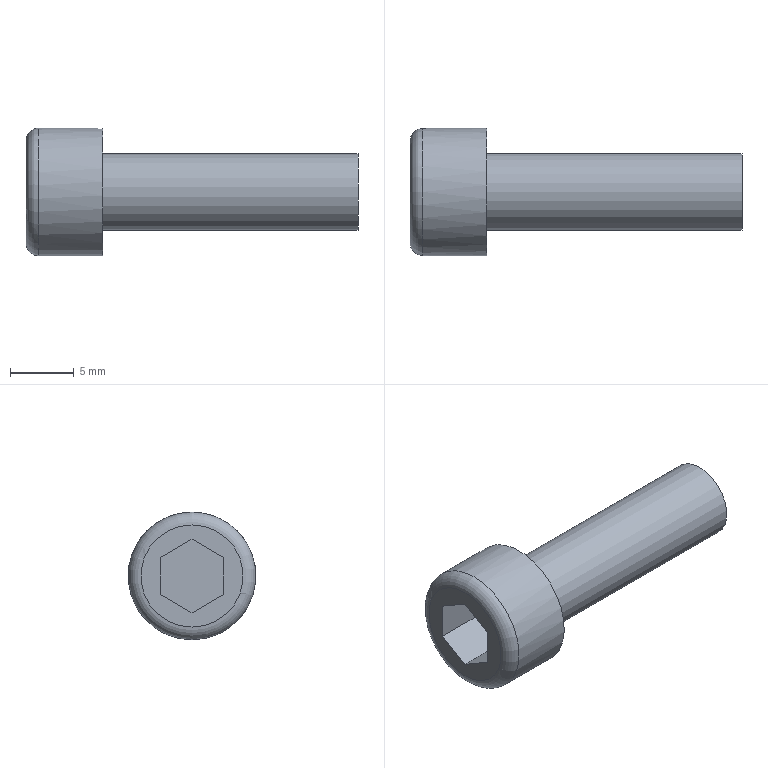Part | STEP file | Tube necking machine_id226_x_t | 1 solid | 13 faces | box 26 x 10 x 10 mm | volume 944.548 mm3 | plane 10 | cylinder 2 | torus 1 | commonest cylinder face diameters 6 x1 10 x1
STEP:
#1=CARTESIAN_POINT('',(0.,0.,0.));
#2=DIRECTION('',(0.,0.,1.));
#3=DIRECTION('',(1.,0.,0.));
#4=AXIS2_PLACEMENT_3D('',#1,#2,#3);
#5=CARTESIAN_POINT('',(-132.5,-117.,264.));
#6=VERTEX_POINT('',#5);
#7=CARTESIAN_POINT('',(-132.5,-117.,260.));
#8=DIRECTION('',(-1.,0.,0.));
#9=DIRECTION('',(0.,0.,1.));
#10=AXIS2_PLACEMENT_3D('',#7,#8,#9);
#11=CIRCLE('',#10,4.);
#12=CARTESIAN_POINT('',(-132.5,-117.,255.));
#13=DIRECTION('',(1.,0.,0.));
#14=DIRECTION('',(0.,0.,1.));
#15=AXIS2_PLACEMENT_3D('',#12,#13,#14);
#16=PLANE('',#15);
#17=CARTESIAN_POINT('',(9.,0.));
#18=CARTESIAN_POINT('',(9.,-6.928));
#19=CARTESIAN_POINT('',(3.,-3.464));
#20=CARTESIAN_POINT('',(-3.,0.));
#21=CARTESIAN_POINT('',(3.,3.464));
#22=CARTESIAN_POINT('',(9.,6.928));
#23=CARTESIAN_POINT('',(9.,0.));
#24=(BOUNDED_CURVE()B_SPLINE_CURVE(2,(#17,#18,#19,#20,#21,#22,#23),.UNSPECIFIED.,.T.,.F.)B_SPLINE_CURVE_WITH_KNOTS((1,2,2,2,2,1),(-2.094,0.,2.094,4.189,6.283,8.378),.UNSPECIFIED.)CURVE()GEOMETRIC_REPRESENTATION_ITEM()RATIONAL_B_SPLINE_CURVE((1.,0.5,1.,0.5,1.,0.5,1.))REPRESENTATION_ITEM(''));
#25=(GEOMETRIC_REPRESENTATION_CONTEXT(2)PARAMETRIC_REPRESENTATION_CONTEXT()REPRESENTATION_CONTEXT('',''));
#26=DEFINITIONAL_REPRESENTATION('',(#24),#25);
#27=PCURVE('',#16,#26);
#28=CARTESIAN_POINT('',(-131.5,-117.,260.));
#29=DIRECTION('',(1.,0.,0.));
#30=DIRECTION('',(0.,0.,1.));
#31=AXIS2_PLACEMENT_3D('',#28,#29,#30);
#32=TOROIDAL_SURFACE('',#31,4.,1.);
#33=CARTESIAN_POINT('',(6.283,4.712));
#34=DIRECTION('',(-1.,0.));
#35=VECTOR('',#34,1.);
#36=LINE('',#33,#35);
#37=(GEOMETRIC_REPRESENTATION_CONTEXT(2)PARAMETRIC_REPRESENTATION_CONTEXT()REPRESENTATION_CONTEXT('',''));
#38=DEFINITIONAL_REPRESENTATION('',(#36),#37);
#39=PCURVE('',#32,#38);
#40=SURFACE_CURVE('',#11,(#27,#39),.PCURVE_S1.);
#41=EDGE_CURVE('',#6,#6,#40,.T.);
#42=ORIENTED_EDGE('',*,*,#41,.T.);
#43=EDGE_LOOP('',(#42));
#44=FACE_BOUND('',#43,.T.);
#45=CARTESIAN_POINT('',(-132.5,-114.5,258.557));
#46=VERTEX_POINT('',#45);
#47=CARTESIAN_POINT('',(-132.5,-114.5,261.443));
#48=VERTEX_POINT('',#47);
#49=CARTESIAN_POINT('',(-132.5,-114.5,261.443));
#50=DIRECTION('',(0.,0.,1.));
#51=VECTOR('',#50,1.);
#52=LINE('',#49,#51);
#53=CARTESIAN_POINT('',(6.443,-2.5));
#54=DIRECTION('',(1.,0.));
#55=VECTOR('',#54,1.);
#56=LINE('',#53,#55);
#57=(GEOMETRIC_REPRESENTATION_CONTEXT(2)PARAMETRIC_REPRESENTATION_CONTEXT()REPRESENTATION_CONTEXT('',''));
#58=DEFINITIONAL_REPRESENTATION('',(#56),#57);
#59=PCURVE('',#16,#58);
#60=CARTESIAN_POINT('',(-128.54,-114.5,261.443));
#61=DIRECTION('',(0.,-1.,0.));
#62=DIRECTION('',(1.,0.,0.));
#63=AXIS2_PLACEMENT_3D('',#60,#61,#62);
#64=PLANE('',#63);
#65=CARTESIAN_POINT('',(-3.96,0.));
#66=DIRECTION('',(0.,1.));
#67=VECTOR('',#66,1.);
#68=LINE('',#65,#67);
#69=(GEOMETRIC_REPRESENTATION_CONTEXT(2)PARAMETRIC_REPRESENTATION_CONTEXT()REPRESENTATION_CONTEXT('',''));
#70=DEFINITIONAL_REPRESENTATION('',(#68),#69);
#71=PCURVE('',#64,#70);
#72=SURFACE_CURVE('',#52,(#59,#71),.PCURVE_S1.);
#73=EDGE_CURVE('',#46,#48,#72,.T.);
#74=ORIENTED_EDGE('',*,*,#73,.T.);
#75=CARTESIAN_POINT('',(-132.5,-117.,262.887));
#76=VERTEX_POINT('',#75);
#77=CARTESIAN_POINT('',(-132.5,-117.,262.887));
#78=DIRECTION('',(0.,-0.866,0.5));
#79=VECTOR('',#78,1.);
#80=LINE('',#77,#79);
#81=CARTESIAN_POINT('',(7.887,0.));
#82=DIRECTION('',(0.5,0.866));
#83=VECTOR('',#82,1.);
#84=LINE('',#81,#83);
#85=(GEOMETRIC_REPRESENTATION_CONTEXT(2)PARAMETRIC_REPRESENTATION_CONTEXT()REPRESENTATION_CONTEXT('',''));
#86=DEFINITIONAL_REPRESENTATION('',(#84),#85);
#87=PCURVE('',#16,#86);
#88=CARTESIAN_POINT('',(-128.54,-117.,262.887));
#89=DIRECTION('',(0.,-0.5,-0.866));
#90=DIRECTION('',(0.,0.866,-0.5));
#91=AXIS2_PLACEMENT_3D('',#88,#89,#90);
#92=PLANE('',#91);
#93=CARTESIAN_POINT('',(0.,-3.96));
#94=DIRECTION('',(-1.,0.));
#95=VECTOR('',#94,1.);
#96=LINE('',#93,#95);
#97=(GEOMETRIC_REPRESENTATION_CONTEXT(2)PARAMETRIC_REPRESENTATION_CONTEXT()REPRESENTATION_CONTEXT('',''));
#98=DEFINITIONAL_REPRESENTATION('',(#96),#97);
#99=PCURVE('',#92,#98);
#100=SURFACE_CURVE('',#80,(#87,#99),.PCURVE_S1.);
#101=EDGE_CURVE('',#48,#76,#100,.T.);
#102=ORIENTED_EDGE('',*,*,#101,.T.);
#103=CARTESIAN_POINT('',(-132.5,-119.5,261.443));
#104=VERTEX_POINT('',#103);
#105=CARTESIAN_POINT('',(-132.5,-119.5,261.443));
#106=DIRECTION('',(0.,-0.866,-0.5));
#107=VECTOR('',#106,1.);
#108=LINE('',#105,#107);
#109=CARTESIAN_POINT('',(6.443,2.5));
#110=DIRECTION('',(-0.5,0.866));
#111=VECTOR('',#110,1.);
#112=LINE('',#109,#111);
#113=(GEOMETRIC_REPRESENTATION_CONTEXT(2)PARAMETRIC_REPRESENTATION_CONTEXT()REPRESENTATION_CONTEXT('',''));
#114=DEFINITIONAL_REPRESENTATION('',(#112),#113);
#115=PCURVE('',#16,#114);
#116=CARTESIAN_POINT('',(-128.54,-119.5,261.443));
#117=DIRECTION('',(0.,0.5,-0.866));
#118=DIRECTION('',(0.,0.866,0.5));
#119=AXIS2_PLACEMENT_3D('',#116,#117,#118);
#120=PLANE('',#119);
#121=CARTESIAN_POINT('',(0.,-3.96));
#122=DIRECTION('',(-1.,0.));
#123=VECTOR('',#122,1.);
#124=LINE('',#121,#123);
#125=(GEOMETRIC_REPRESENTATION_CONTEXT(2)PARAMETRIC_REPRESENTATION_CONTEXT()REPRESENTATION_CONTEXT('',''));
#126=DEFINITIONAL_REPRESENTATION('',(#124),#125);
#127=PCURVE('',#120,#126);
#128=SURFACE_CURVE('',#108,(#115,#127),.PCURVE_S1.);
#129=EDGE_CURVE('',#76,#104,#128,.T.);
#130=ORIENTED_EDGE('',*,*,#129,.T.);
#131=CARTESIAN_POINT('',(-132.5,-119.5,258.557));
#132=VERTEX_POINT('',#131);
#133=CARTESIAN_POINT('',(-132.5,-119.5,258.557));
#134=DIRECTION('',(0.,0.,-1.));
#135=VECTOR('',#134,1.);
#136=LINE('',#133,#135);
#137=CARTESIAN_POINT('',(3.557,2.5));
#138=DIRECTION('',(-1.,0.));
#139=VECTOR('',#138,1.);
#140=LINE('',#137,#139);
#141=(GEOMETRIC_REPRESENTATION_CONTEXT(2)PARAMETRIC_REPRESENTATION_CONTEXT()REPRESENTATION_CONTEXT('',''));
#142=DEFINITIONAL_REPRESENTATION('',(#140),#141);
#143=PCURVE('',#16,#142);
#144=CARTESIAN_POINT('',(-128.54,-119.5,258.557));
#145=DIRECTION('',(0.,1.,0.));
#146=DIRECTION('',(0.,0.,1.));
#147=AXIS2_PLACEMENT_3D('',#144,#145,#146);
#148=PLANE('',#147);
#149=CARTESIAN_POINT('',(0.,-3.96));
#150=DIRECTION('',(-1.,0.));
#151=VECTOR('',#150,1.);
#152=LINE('',#149,#151);
#153=(GEOMETRIC_REPRESENTATION_CONTEXT(2)PARAMETRIC_REPRESENTATION_CONTEXT()REPRESENTATION_CONTEXT('',''));
#154=DEFINITIONAL_REPRESENTATION('',(#152),#153);
#155=PCURVE('',#148,#154);
#156=SURFACE_CURVE('',#136,(#143,#155),.PCURVE_S1.);
#157=EDGE_CURVE('',#104,#132,#156,.T.);
#158=ORIENTED_EDGE('',*,*,#157,.T.);
#159=CARTESIAN_POINT('',(-132.5,-117.,257.113));
#160=VERTEX_POINT('',#159);
#161=CARTESIAN_POINT('',(-132.5,-117.,257.113));
#162=DIRECTION('',(0.,0.866,-0.5));
#163=VECTOR('',#162,1.);
#164=LINE('',#161,#163);
#165=CARTESIAN_POINT('',(2.113,0.));
#166=DIRECTION('',(-0.5,-0.866));
#167=VECTOR('',#166,1.);
#168=LINE('',#165,#167);
#169=(GEOMETRIC_REPRESENTATION_CONTEXT(2)PARAMETRIC_REPRESENTATION_CONTEXT()REPRESENTATION_CONTEXT('',''));
#170=DEFINITIONAL_REPRESENTATION('',(#168),#169);
#171=PCURVE('',#16,#170);
#172=CARTESIAN_POINT('',(-128.54,-117.,257.113));
#173=DIRECTION('',(0.,0.5,0.866));
#174=DIRECTION('',(0.,-0.866,0.5));
#175=AXIS2_PLACEMENT_3D('',#172,#173,#174);
#176=PLANE('',#175);
#177=CARTESIAN_POINT('',(0.,-3.96));
#178=DIRECTION('',(-1.,0.));
#179=VECTOR('',#178,1.);
#180=LINE('',#177,#179);
#181=(GEOMETRIC_REPRESENTATION_CONTEXT(2)PARAMETRIC_REPRESENTATION_CONTEXT()REPRESENTATION_CONTEXT('',''));
#182=DEFINITIONAL_REPRESENTATION('',(#180),#181);
#183=PCURVE('',#176,#182);
#184=SURFACE_CURVE('',#164,(#171,#183),.PCURVE_S1.);
#185=EDGE_CURVE('',#132,#160,#184,.T.);
#186=ORIENTED_EDGE('',*,*,#185,.T.);
#187=CARTESIAN_POINT('',(-132.5,-114.5,258.557));
#188=DIRECTION('',(0.,0.866,0.5));
#189=VECTOR('',#188,1.);
#190=LINE('',#187,#189);
#191=CARTESIAN_POINT('',(3.557,-2.5));
#192=DIRECTION('',(0.5,-0.866));
#193=VECTOR('',#192,1.);
#194=LINE('',#191,#193);
#195=(GEOMETRIC_REPRESENTATION_CONTEXT(2)PARAMETRIC_REPRESENTATION_CONTEXT()REPRESENTATION_CONTEXT('',''));
#196=DEFINITIONAL_REPRESENTATION('',(#194),#195);
#197=PCURVE('',#16,#196);
#198=CARTESIAN_POINT('',(-128.54,-114.5,258.557));
#199=DIRECTION('',(0.,-0.5,0.866));
#200=DIRECTION('',(0.,-0.866,-0.5));
#201=AXIS2_PLACEMENT_3D('',#198,#199,#200);
#202=PLANE('',#201);
#203=CARTESIAN_POINT('',(0.,-3.96));
#204=DIRECTION('',(-1.,0.));
#205=VECTOR('',#204,1.);
#206=LINE('',#203,#205);
#207=(GEOMETRIC_REPRESENTATION_CONTEXT(2)PARAMETRIC_REPRESENTATION_CONTEXT()REPRESENTATION_CONTEXT('',''));
#208=DEFINITIONAL_REPRESENTATION('',(#206),#207);
#209=PCURVE('',#202,#208);
#210=SURFACE_CURVE('',#190,(#197,#209),.PCURVE_S1.);
#211=EDGE_CURVE('',#160,#46,#210,.T.);
#212=ORIENTED_EDGE('',*,*,#211,.T.);
#213=EDGE_LOOP('',(#74,#102,#130,#158,#186,#212));
#214=FACE_BOUND('',#213,.T.);
#215=ADVANCED_FACE('',(#44,#214),#16,.F.);
#216=CARTESIAN_POINT('',(-131.5,-117.,265.));
#217=VERTEX_POINT('',#216);
#218=CARTESIAN_POINT('',(-131.5,-117.,255.));
#219=VERTEX_POINT('',#218);
#220=CARTESIAN_POINT('',(-131.5,-117.,260.));
#221=DIRECTION('',(1.,0.,0.));
#222=DIRECTION('',(0.,0.,1.));
#223=AXIS2_PLACEMENT_3D('',#220,#221,#222);
#224=CIRCLE('',#223,5.);
#225=CARTESIAN_POINT('',(-127.6,-117.,260.));
#226=DIRECTION('',(-1.,0.,0.));
#227=DIRECTION('',(0.,0.,-1.));
#228=AXIS2_PLACEMENT_3D('',#225,#226,#227);
#229=CYLINDRICAL_SURFACE('',#228,5.);
#230=CARTESIAN_POINT('',(3.142,3.9));
#231=DIRECTION('',(-1.,0.));
#232=VECTOR('',#231,1.);
#233=LINE('',#230,#232);
#234=(GEOMETRIC_REPRESENTATION_CONTEXT(2)PARAMETRIC_REPRESENTATION_CONTEXT()REPRESENTATION_CONTEXT('',''));
#235=DEFINITIONAL_REPRESENTATION('',(#233),#234);
#236=PCURVE('',#229,#235);
#237=CARTESIAN_POINT('',(0.,6.283));
#238=DIRECTION('',(1.,0.));
#239=VECTOR('',#238,1.);
#240=LINE('',#237,#239);
#241=(GEOMETRIC_REPRESENTATION_CONTEXT(2)PARAMETRIC_REPRESENTATION_CONTEXT()REPRESENTATION_CONTEXT('',''));
#242=DEFINITIONAL_REPRESENTATION('',(#240),#241);
#243=PCURVE('',#32,#242);
#244=SURFACE_CURVE('',#224,(#236,#243),.PCURVE_S1.);
#245=EDGE_CURVE('',#217,#219,#244,.T.);
#246=ORIENTED_EDGE('',*,*,#245,.T.);
#247=CARTESIAN_POINT('',(-126.5,-117.,255.));
#248=VERTEX_POINT('',#247);
#249=CARTESIAN_POINT('',(-126.5,-117.,255.));
#250=CARTESIAN_POINT('',(-131.5,-117.,255.));
#251=B_SPLINE_CURVE_WITH_KNOTS('',1,(#249,#250),.UNSPECIFIED.,.F.,.F.,(2,2),(-1.1,3.9),.PIECEWISE_BEZIER_KNOTS.);
#252=CARTESIAN_POINT('',(0.,0.));
#253=DIRECTION('',(0.,1.));
#254=VECTOR('',#253,1.);
#255=LINE('',#252,#254);
#256=(GEOMETRIC_REPRESENTATION_CONTEXT(2)PARAMETRIC_REPRESENTATION_CONTEXT()REPRESENTATION_CONTEXT('',''));
#257=DEFINITIONAL_REPRESENTATION('',(#255),#256);
#258=PCURVE('',#229,#257);
#259=CARTESIAN_POINT('',(6.283,0.));
#260=DIRECTION('',(0.,1.));
#261=VECTOR('',#260,1.);
#262=LINE('',#259,#261);
#263=(GEOMETRIC_REPRESENTATION_CONTEXT(2)PARAMETRIC_REPRESENTATION_CONTEXT()REPRESENTATION_CONTEXT('',''));
#264=DEFINITIONAL_REPRESENTATION('',(#262),#263);
#265=PCURVE('',#229,#264);
#266=SEAM_CURVE('',#251,(#258,#265),.PCURVE_S1.);
#267=EDGE_CURVE('',#248,#219,#266,.T.);
#268=ORIENTED_EDGE('',*,*,#267,.F.);
#269=CARTESIAN_POINT('',(-126.5,-117.,260.));
#270=DIRECTION('',(-1.,0.,0.));
#271=DIRECTION('',(0.,0.,-1.));
#272=AXIS2_PLACEMENT_3D('',#269,#270,#271);
#273=CIRCLE('',#272,5.);
#274=CARTESIAN_POINT('',(0.,-1.1));
#275=DIRECTION('',(1.,0.));
#276=VECTOR('',#275,1.);
#277=LINE('',#274,#276);
#278=(GEOMETRIC_REPRESENTATION_CONTEXT(2)PARAMETRIC_REPRESENTATION_CONTEXT()REPRESENTATION_CONTEXT('',''));
#279=DEFINITIONAL_REPRESENTATION('',(#277),#278);
#280=PCURVE('',#229,#279);
#281=CARTESIAN_POINT('',(-126.5,-117.,257.));
#282=DIRECTION('',(-1.,0.,0.));
#283=DIRECTION('',(0.,0.,-1.));
#284=AXIS2_PLACEMENT_3D('',#281,#282,#283);
#285=PLANE('',#284);
#286=CARTESIAN_POINT('',(-3.,0.));
#287=DIRECTION('',(1.,0.));
#288=AXIS2_PLACEMENT_2D('',#286,#287);
#289=CIRCLE('',#288,5.);
#290=(GEOMETRIC_REPRESENTATION_CONTEXT(2)PARAMETRIC_REPRESENTATION_CONTEXT()REPRESENTATION_CONTEXT('',''));
#291=DEFINITIONAL_REPRESENTATION('',(#289),#290);
#292=PCURVE('',#285,#291);
#293=SURFACE_CURVE('',#273,(#280,#292),.PCURVE_S1.);
#294=EDGE_CURVE('',#248,#248,#293,.T.);
#295=ORIENTED_EDGE('',*,*,#294,.T.);
#296=ORIENTED_EDGE('',*,*,#267,.T.);
#297=CARTESIAN_POINT('',(-131.5,-117.,260.));
#298=DIRECTION('',(1.,0.,0.));
#299=DIRECTION('',(0.,0.,1.));
#300=AXIS2_PLACEMENT_3D('',#297,#298,#299);
#301=CIRCLE('',#300,5.);
#302=CARTESIAN_POINT('',(9.425,3.9));
#303=DIRECTION('',(-1.,0.));
#304=VECTOR('',#303,1.);
#305=LINE('',#302,#304);
#306=(GEOMETRIC_REPRESENTATION_CONTEXT(2)PARAMETRIC_REPRESENTATION_CONTEXT()REPRESENTATION_CONTEXT('',''));
#307=DEFINITIONAL_REPRESENTATION('',(#305),#306);
#308=PCURVE('',#229,#307);
#309=CARTESIAN_POINT('',(0.,6.283));
#310=DIRECTION('',(1.,0.));
#311=VECTOR('',#310,1.);
#312=LINE('',#309,#311);
#313=(GEOMETRIC_REPRESENTATION_CONTEXT(2)PARAMETRIC_REPRESENTATION_CONTEXT()REPRESENTATION_CONTEXT('',''));
#314=DEFINITIONAL_REPRESENTATION('',(#312),#313);
#315=PCURVE('',#32,#314);
#316=SURFACE_CURVE('',#301,(#308,#315),.PCURVE_S1.);
#317=EDGE_CURVE('',#219,#217,#316,.T.);
#318=ORIENTED_EDGE('',*,*,#317,.T.);
#319=EDGE_LOOP('',(#246,#268,#295,#296,#318));
#320=FACE_BOUND('',#319,.T.);
#321=ADVANCED_FACE('',(#320),#229,.T.);
#322=ORIENTED_EDGE('',*,*,#294,.F.);
#323=EDGE_LOOP('',(#322));
#324=FACE_BOUND('',#323,.T.);
#325=CARTESIAN_POINT('',(-126.5,-117.,257.));
#326=VERTEX_POINT('',#325);
#327=CARTESIAN_POINT('',(-126.5,-117.,260.));
#328=DIRECTION('',(-1.,0.,0.));
#329=DIRECTION('',(0.,0.,-1.));
#330=AXIS2_PLACEMENT_3D('',#327,#328,#329);
#331=CIRCLE('',#330,3.);
#332=CARTESIAN_POINT('',(-3.,0.));
#333=DIRECTION('',(1.,0.));
#334=AXIS2_PLACEMENT_2D('',#332,#333);
#335=CIRCLE('',#334,3.);
#336=(GEOMETRIC_REPRESENTATION_CONTEXT(2)PARAMETRIC_REPRESENTATION_CONTEXT()REPRESENTATION_CONTEXT('',''));
#337=DEFINITIONAL_REPRESENTATION('',(#335),#336);
#338=PCURVE('',#285,#337);
#339=CARTESIAN_POINT('',(-127.6,-117.,260.));
#340=DIRECTION('',(-1.,0.,0.));
#341=DIRECTION('',(0.,0.,-1.));
#342=AXIS2_PLACEMENT_3D('',#339,#340,#341);
#343=CYLINDRICAL_SURFACE('',#342,3.);
#344=CARTESIAN_POINT('',(0.,-1.1));
#345=DIRECTION('',(1.,0.));
#346=VECTOR('',#345,1.);
#347=LINE('',#344,#346);
#348=(GEOMETRIC_REPRESENTATION_CONTEXT(2)PARAMETRIC_REPRESENTATION_CONTEXT()REPRESENTATION_CONTEXT('',''));
#349=DEFINITIONAL_REPRESENTATION('',(#347),#348);
#350=PCURVE('',#343,#349);
#351=SURFACE_CURVE('',#331,(#338,#350),.PCURVE_S1.);
#352=EDGE_CURVE('',#326,#326,#351,.T.);
#353=ORIENTED_EDGE('',*,*,#352,.T.);
#354=EDGE_LOOP('',(#353));
#355=FACE_BOUND('',#354,.T.);
#356=ADVANCED_FACE('',(#324,#355),#285,.F.);
#357=ORIENTED_EDGE('',*,*,#352,.F.);
#358=CARTESIAN_POINT('',(-106.5,-117.,257.));
#359=VERTEX_POINT('',#358);
#360=CARTESIAN_POINT('',(-106.5,-117.,257.));
#361=CARTESIAN_POINT('',(-126.5,-117.,257.));
#362=B_SPLINE_CURVE_WITH_KNOTS('',1,(#360,#361),.UNSPECIFIED.,.F.,.F.,(2,2),(-21.1,-1.1),.PIECEWISE_BEZIER_KNOTS.);
#363=CARTESIAN_POINT('',(0.,0.));
#364=DIRECTION('',(0.,1.));
#365=VECTOR('',#364,1.);
#366=LINE('',#363,#365);
#367=(GEOMETRIC_REPRESENTATION_CONTEXT(2)PARAMETRIC_REPRESENTATION_CONTEXT()REPRESENTATION_CONTEXT('',''));
#368=DEFINITIONAL_REPRESENTATION('',(#366),#367);
#369=PCURVE('',#343,#368);
#370=CARTESIAN_POINT('',(6.283,0.));
#371=DIRECTION('',(0.,1.));
#372=VECTOR('',#371,1.);
#373=LINE('',#370,#372);
#374=(GEOMETRIC_REPRESENTATION_CONTEXT(2)PARAMETRIC_REPRESENTATION_CONTEXT()REPRESENTATION_CONTEXT('',''));
#375=DEFINITIONAL_REPRESENTATION('',(#373),#374);
#376=PCURVE('',#343,#375);
#377=SEAM_CURVE('',#362,(#369,#376),.PCURVE_S1.);
#378=EDGE_CURVE('',#359,#326,#377,.T.);
#379=ORIENTED_EDGE('',*,*,#378,.F.);
#380=CARTESIAN_POINT('',(-106.5,-117.,260.));
#381=DIRECTION('',(-1.,0.,0.));
#382=DIRECTION('',(0.,0.,-1.));
#383=AXIS2_PLACEMENT_3D('',#380,#381,#382);
#384=CIRCLE('',#383,3.);
#385=CARTESIAN_POINT('',(0.,-21.1));
#386=DIRECTION('',(1.,0.));
#387=VECTOR('',#386,1.);
#388=LINE('',#385,#387);
#389=(GEOMETRIC_REPRESENTATION_CONTEXT(2)PARAMETRIC_REPRESENTATION_CONTEXT()REPRESENTATION_CONTEXT('',''));
#390=DEFINITIONAL_REPRESENTATION('',(#388),#389);
#391=PCURVE('',#343,#390);
#392=CARTESIAN_POINT('',(-106.5,-117.,260.));
#393=DIRECTION('',(-1.,0.,0.));
#394=DIRECTION('',(0.,0.,-1.));
#395=AXIS2_PLACEMENT_3D('',#392,#393,#394);
#396=PLANE('',#395);
#397=CARTESIAN_POINT('',(0.,0.));
#398=DIRECTION('',(1.,0.));
#399=AXIS2_PLACEMENT_2D('',#397,#398);
#400=CIRCLE('',#399,3.);
#401=(GEOMETRIC_REPRESENTATION_CONTEXT(2)PARAMETRIC_REPRESENTATION_CONTEXT()REPRESENTATION_CONTEXT('',''));
#402=DEFINITIONAL_REPRESENTATION('',(#400),#401);
#403=PCURVE('',#396,#402);
#404=SURFACE_CURVE('',#384,(#391,#403),.PCURVE_S1.);
#405=EDGE_CURVE('',#359,#359,#404,.T.);
#406=ORIENTED_EDGE('',*,*,#405,.T.);
#407=ORIENTED_EDGE('',*,*,#378,.T.);
#408=EDGE_LOOP('',(#357,#379,#406,#407));
#409=FACE_BOUND('',#408,.T.);
#410=ADVANCED_FACE('',(#409),#343,.T.);
#411=ORIENTED_EDGE('',*,*,#405,.F.);
#412=EDGE_LOOP('',(#411));
#413=FACE_BOUND('',#412,.T.);
#414=ADVANCED_FACE('',(#413),#396,.F.);
#415=ORIENTED_EDGE('',*,*,#73,.F.);
#416=CARTESIAN_POINT('',(-128.54,-114.5,258.557));
#417=VERTEX_POINT('',#416);
#418=CARTESIAN_POINT('',(-128.54,-114.5,258.557));
#419=DIRECTION('',(-1.,0.,0.));
#420=VECTOR('',#419,1.);
#421=LINE('',#418,#420);
#422=CARTESIAN_POINT('',(0.,-2.887));
#423=DIRECTION('',(-1.,0.));
#424=VECTOR('',#423,1.);
#425=LINE('',#422,#424);
#426=(GEOMETRIC_REPRESENTATION_CONTEXT(2)PARAMETRIC_REPRESENTATION_CONTEXT()REPRESENTATION_CONTEXT('',''));
#427=DEFINITIONAL_REPRESENTATION('',(#425),#426);
#428=PCURVE('',#64,#427);
#429=CARTESIAN_POINT('',(0.,0.));
#430=DIRECTION('',(0.,-1.));
#431=VECTOR('',#430,1.);
#432=LINE('',#429,#431);
#433=(GEOMETRIC_REPRESENTATION_CONTEXT(2)PARAMETRIC_REPRESENTATION_CONTEXT()REPRESENTATION_CONTEXT('',''));
#434=DEFINITIONAL_REPRESENTATION('',(#432),#433);
#435=PCURVE('',#202,#434);
#436=SURFACE_CURVE('',#421,(#428,#435),.PCURVE_S1.);
#437=EDGE_CURVE('',#417,#46,#436,.T.);
#438=ORIENTED_EDGE('',*,*,#437,.F.);
#439=CARTESIAN_POINT('',(-128.54,-114.5,261.443));
#440=VERTEX_POINT('',#439);
#441=CARTESIAN_POINT('',(-128.54,-114.5,261.443));
#442=DIRECTION('',(0.,0.,-1.));
#443=VECTOR('',#442,1.);
#444=LINE('',#441,#443);
#445=CARTESIAN_POINT('',(0.,0.));
#446=DIRECTION('',(0.,-1.));
#447=VECTOR('',#446,1.);
#448=LINE('',#445,#447);
#449=(GEOMETRIC_REPRESENTATION_CONTEXT(2)PARAMETRIC_REPRESENTATION_CONTEXT()REPRESENTATION_CONTEXT('',''));
#450=DEFINITIONAL_REPRESENTATION('',(#448),#449);
#451=PCURVE('',#64,#450);
#452=CARTESIAN_POINT('',(-128.54,-117.,260.));
#453=DIRECTION('',(1.,0.,0.));
#454=DIRECTION('',(0.,0.,1.));
#455=AXIS2_PLACEMENT_3D('',#452,#453,#454);
#456=PLANE('',#455);
#457=CARTESIAN_POINT('',(1.443,-2.5));
#458=DIRECTION('',(-1.,0.));
#459=VECTOR('',#458,1.);
#460=LINE('',#457,#459);
#461=(GEOMETRIC_REPRESENTATION_CONTEXT(2)PARAMETRIC_REPRESENTATION_CONTEXT()REPRESENTATION_CONTEXT('',''));
#462=DEFINITIONAL_REPRESENTATION('',(#460),#461);
#463=PCURVE('',#456,#462);
#464=SURFACE_CURVE('',#444,(#451,#463),.PCURVE_S1.);
#465=EDGE_CURVE('',#440,#417,#464,.T.);
#466=ORIENTED_EDGE('',*,*,#465,.F.);
#467=CARTESIAN_POINT('',(-128.54,-114.5,261.443));
#468=DIRECTION('',(-1.,0.,0.));
#469=VECTOR('',#468,1.);
#470=LINE('',#467,#469);
#471=CARTESIAN_POINT('',(0.,0.));
#472=DIRECTION('',(-1.,0.));
#473=VECTOR('',#472,1.);
#474=LINE('',#471,#473);
#475=(GEOMETRIC_REPRESENTATION_CONTEXT(2)PARAMETRIC_REPRESENTATION_CONTEXT()REPRESENTATION_CONTEXT('',''));
#476=DEFINITIONAL_REPRESENTATION('',(#474),#475);
#477=PCURVE('',#64,#476);
#478=CARTESIAN_POINT('',(2.887,0.));
#479=DIRECTION('',(0.,-1.));
#480=VECTOR('',#479,1.);
#481=LINE('',#478,#480);
#482=(GEOMETRIC_REPRESENTATION_CONTEXT(2)PARAMETRIC_REPRESENTATION_CONTEXT()REPRESENTATION_CONTEXT('',''));
#483=DEFINITIONAL_REPRESENTATION('',(#481),#482);
#484=PCURVE('',#92,#483);
#485=SURFACE_CURVE('',#470,(#477,#484),.PCURVE_S1.);
#486=EDGE_CURVE('',#440,#48,#485,.T.);
#487=ORIENTED_EDGE('',*,*,#486,.T.);
#488=EDGE_LOOP('',(#415,#438,#466,#487));
#489=FACE_BOUND('',#488,.T.);
#490=ADVANCED_FACE('',(#489),#64,.T.);
#491=ORIENTED_EDGE('',*,*,#211,.F.);
#492=CARTESIAN_POINT('',(-128.54,-117.,257.113));
#493=VERTEX_POINT('',#492);
#494=CARTESIAN_POINT('',(-128.54,-117.,257.113));
#495=DIRECTION('',(-1.,0.,0.));
#496=VECTOR('',#495,1.);
#497=LINE('',#494,#496);
#498=CARTESIAN_POINT('',(2.887,0.));
#499=DIRECTION('',(0.,-1.));
#500=VECTOR('',#499,1.);
#501=LINE('',#498,#500);
#502=(GEOMETRIC_REPRESENTATION_CONTEXT(2)PARAMETRIC_REPRESENTATION_CONTEXT()REPRESENTATION_CONTEXT('',''));
#503=DEFINITIONAL_REPRESENTATION('',(#501),#502);
#504=PCURVE('',#202,#503);
#505=CARTESIAN_POINT('',(0.,0.));
#506=DIRECTION('',(0.,-1.));
#507=VECTOR('',#506,1.);
#508=LINE('',#505,#507);
#509=(GEOMETRIC_REPRESENTATION_CONTEXT(2)PARAMETRIC_REPRESENTATION_CONTEXT()REPRESENTATION_CONTEXT('',''));
#510=DEFINITIONAL_REPRESENTATION('',(#508),#509);
#511=PCURVE('',#176,#510);
#512=SURFACE_CURVE('',#497,(#504,#511),.PCURVE_S1.);
#513=EDGE_CURVE('',#493,#160,#512,.T.);
#514=ORIENTED_EDGE('',*,*,#513,.F.);
#515=CARTESIAN_POINT('',(-128.54,-114.5,258.557));
#516=DIRECTION('',(0.,-0.866,-0.5));
#517=VECTOR('',#516,1.);
#518=LINE('',#515,#517);
#519=CARTESIAN_POINT('',(0.,0.));
#520=DIRECTION('',(1.,0.));
#521=VECTOR('',#520,1.);
#522=LINE('',#519,#521);
#523=(GEOMETRIC_REPRESENTATION_CONTEXT(2)PARAMETRIC_REPRESENTATION_CONTEXT()REPRESENTATION_CONTEXT('',''));
#524=DEFINITIONAL_REPRESENTATION('',(#522),#523);
#525=PCURVE('',#202,#524);
#526=CARTESIAN_POINT('',(-1.443,-2.5));
#527=DIRECTION('',(-0.5,0.866));
#528=VECTOR('',#527,1.);
#529=LINE('',#526,#528);
#530=(GEOMETRIC_REPRESENTATION_CONTEXT(2)PARAMETRIC_REPRESENTATION_CONTEXT()REPRESENTATION_CONTEXT('',''));
#531=DEFINITIONAL_REPRESENTATION('',(#529),#530);
#532=PCURVE('',#456,#531);
#533=SURFACE_CURVE('',#518,(#525,#532),.PCURVE_S1.);
#534=EDGE_CURVE('',#417,#493,#533,.T.);
#535=ORIENTED_EDGE('',*,*,#534,.F.);
#536=ORIENTED_EDGE('',*,*,#437,.T.);
#537=EDGE_LOOP('',(#491,#514,#535,#536));
#538=FACE_BOUND('',#537,.T.);
#539=ADVANCED_FACE('',(#538),#202,.T.);
#540=ORIENTED_EDGE('',*,*,#185,.F.);
#541=CARTESIAN_POINT('',(-128.54,-119.5,258.557));
#542=VERTEX_POINT('',#541);
#543=CARTESIAN_POINT('',(-128.54,-119.5,258.557));
#544=DIRECTION('',(-1.,0.,0.));
#545=VECTOR('',#544,1.);
#546=LINE('',#543,#545);
#547=CARTESIAN_POINT('',(2.887,0.));
#548=DIRECTION('',(0.,-1.));
#549=VECTOR('',#548,1.);
#550=LINE('',#547,#549);
#551=(GEOMETRIC_REPRESENTATION_CONTEXT(2)PARAMETRIC_REPRESENTATION_CONTEXT()REPRESENTATION_CONTEXT('',''));
#552=DEFINITIONAL_REPRESENTATION('',(#550),#551);
#553=PCURVE('',#176,#552);
#554=CARTESIAN_POINT('',(0.,0.));
#555=DIRECTION('',(0.,-1.));
#556=VECTOR('',#555,1.);
#557=LINE('',#554,#556);
#558=(GEOMETRIC_REPRESENTATION_CONTEXT(2)PARAMETRIC_REPRESENTATION_CONTEXT()REPRESENTATION_CONTEXT('',''));
#559=DEFINITIONAL_REPRESENTATION('',(#557),#558);
#560=PCURVE('',#148,#559);
#561=SURFACE_CURVE('',#546,(#553,#560),.PCURVE_S1.);
#562=EDGE_CURVE('',#542,#132,#561,.T.);
#563=ORIENTED_EDGE('',*,*,#562,.F.);
#564=CARTESIAN_POINT('',(-128.54,-117.,257.113));
#565=DIRECTION('',(0.,-0.866,0.5));
#566=VECTOR('',#565,1.);
#567=LINE('',#564,#566);
#568=CARTESIAN_POINT('',(0.,0.));
#569=DIRECTION('',(1.,0.));
#570=VECTOR('',#569,1.);
#571=LINE('',#568,#570);
#572=(GEOMETRIC_REPRESENTATION_CONTEXT(2)PARAMETRIC_REPRESENTATION_CONTEXT()REPRESENTATION_CONTEXT('',''));
#573=DEFINITIONAL_REPRESENTATION('',(#571),#572);
#574=PCURVE('',#176,#573);
#575=CARTESIAN_POINT('',(-2.887,0.));
#576=DIRECTION('',(0.5,0.866));
#577=VECTOR('',#576,1.);
#578=LINE('',#575,#577);
#579=(GEOMETRIC_REPRESENTATION_CONTEXT(2)PARAMETRIC_REPRESENTATION_CONTEXT()REPRESENTATION_CONTEXT('',''));
#580=DEFINITIONAL_REPRESENTATION('',(#578),#579);
#581=PCURVE('',#456,#580);
#582=SURFACE_CURVE('',#567,(#574,#581),.PCURVE_S1.);
#583=EDGE_CURVE('',#493,#542,#582,.T.);
#584=ORIENTED_EDGE('',*,*,#583,.F.);
#585=ORIENTED_EDGE('',*,*,#513,.T.);
#586=EDGE_LOOP('',(#540,#563,#584,#585));
#587=FACE_BOUND('',#586,.T.);
#588=ADVANCED_FACE('',(#587),#176,.T.);
#589=ORIENTED_EDGE('',*,*,#157,.F.);
#590=CARTESIAN_POINT('',(-128.54,-119.5,261.443));
#591=VERTEX_POINT('',#590);
#592=CARTESIAN_POINT('',(-128.54,-119.5,261.443));
#593=DIRECTION('',(-1.,0.,0.));
#594=VECTOR('',#593,1.);
#595=LINE('',#592,#594);
#596=CARTESIAN_POINT('',(2.887,0.));
#597=DIRECTION('',(0.,-1.));
#598=VECTOR('',#597,1.);
#599=LINE('',#596,#598);
#600=(GEOMETRIC_REPRESENTATION_CONTEXT(2)PARAMETRIC_REPRESENTATION_CONTEXT()REPRESENTATION_CONTEXT('',''));
#601=DEFINITIONAL_REPRESENTATION('',(#599),#600);
#602=PCURVE('',#148,#601);
#603=CARTESIAN_POINT('',(0.,0.));
#604=DIRECTION('',(0.,-1.));
#605=VECTOR('',#604,1.);
#606=LINE('',#603,#605);
#607=(GEOMETRIC_REPRESENTATION_CONTEXT(2)PARAMETRIC_REPRESENTATION_CONTEXT()REPRESENTATION_CONTEXT('',''));
#608=DEFINITIONAL_REPRESENTATION('',(#606),#607);
#609=PCURVE('',#120,#608);
#610=SURFACE_CURVE('',#595,(#602,#609),.PCURVE_S1.);
#611=EDGE_CURVE('',#591,#104,#610,.T.);
#612=ORIENTED_EDGE('',*,*,#611,.F.);
#613=CARTESIAN_POINT('',(-128.54,-119.5,258.557));
#614=DIRECTION('',(0.,0.,1.));
#615=VECTOR('',#614,1.);
#616=LINE('',#613,#615);
#617=CARTESIAN_POINT('',(0.,0.));
#618=DIRECTION('',(1.,0.));
#619=VECTOR('',#618,1.);
#620=LINE('',#617,#619);
#621=(GEOMETRIC_REPRESENTATION_CONTEXT(2)PARAMETRIC_REPRESENTATION_CONTEXT()REPRESENTATION_CONTEXT('',''));
#622=DEFINITIONAL_REPRESENTATION('',(#620),#621);
#623=PCURVE('',#148,#622);
#624=CARTESIAN_POINT('',(-1.443,2.5));
#625=DIRECTION('',(1.,0.));
#626=VECTOR('',#625,1.);
#627=LINE('',#624,#626);
#628=(GEOMETRIC_REPRESENTATION_CONTEXT(2)PARAMETRIC_REPRESENTATION_CONTEXT()REPRESENTATION_CONTEXT('',''));
#629=DEFINITIONAL_REPRESENTATION('',(#627),#628);
#630=PCURVE('',#456,#629);
#631=SURFACE_CURVE('',#616,(#623,#630),.PCURVE_S1.);
#632=EDGE_CURVE('',#542,#591,#631,.T.);
#633=ORIENTED_EDGE('',*,*,#632,.F.);
#634=ORIENTED_EDGE('',*,*,#562,.T.);
#635=EDGE_LOOP('',(#589,#612,#633,#634));
#636=FACE_BOUND('',#635,.T.);
#637=ADVANCED_FACE('',(#636),#148,.T.);
#638=ORIENTED_EDGE('',*,*,#129,.F.);
#639=CARTESIAN_POINT('',(-128.54,-117.,262.887));
#640=VERTEX_POINT('',#639);
#641=CARTESIAN_POINT('',(-128.54,-117.,262.887));
#642=DIRECTION('',(-1.,0.,0.));
#643=VECTOR('',#642,1.);
#644=LINE('',#641,#643);
#645=CARTESIAN_POINT('',(2.887,0.));
#646=DIRECTION('',(0.,-1.));
#647=VECTOR('',#646,1.);
#648=LINE('',#645,#647);
#649=(GEOMETRIC_REPRESENTATION_CONTEXT(2)PARAMETRIC_REPRESENTATION_CONTEXT()REPRESENTATION_CONTEXT('',''));
#650=DEFINITIONAL_REPRESENTATION('',(#648),#649);
#651=PCURVE('',#120,#650);
#652=CARTESIAN_POINT('',(0.,0.));
#653=DIRECTION('',(0.,-1.));
#654=VECTOR('',#653,1.);
#655=LINE('',#652,#654);
#656=(GEOMETRIC_REPRESENTATION_CONTEXT(2)PARAMETRIC_REPRESENTATION_CONTEXT()REPRESENTATION_CONTEXT('',''));
#657=DEFINITIONAL_REPRESENTATION('',(#655),#656);
#658=PCURVE('',#92,#657);
#659=SURFACE_CURVE('',#644,(#651,#658),.PCURVE_S1.);
#660=EDGE_CURVE('',#640,#76,#659,.T.);
#661=ORIENTED_EDGE('',*,*,#660,.F.);
#662=CARTESIAN_POINT('',(-128.54,-119.5,261.443));
#663=DIRECTION('',(0.,0.866,0.5));
#664=VECTOR('',#663,1.);
#665=LINE('',#662,#664);
#666=CARTESIAN_POINT('',(0.,0.));
#667=DIRECTION('',(1.,0.));
#668=VECTOR('',#667,1.);
#669=LINE('',#666,#668);
#670=(GEOMETRIC_REPRESENTATION_CONTEXT(2)PARAMETRIC_REPRESENTATION_CONTEXT()REPRESENTATION_CONTEXT('',''));
#671=DEFINITIONAL_REPRESENTATION('',(#669),#670);
#672=PCURVE('',#120,#671);
#673=CARTESIAN_POINT('',(1.443,2.5));
#674=DIRECTION('',(0.5,-0.866));
#675=VECTOR('',#674,1.);
#676=LINE('',#673,#675);
#677=(GEOMETRIC_REPRESENTATION_CONTEXT(2)PARAMETRIC_REPRESENTATION_CONTEXT()REPRESENTATION_CONTEXT('',''));
#678=DEFINITIONAL_REPRESENTATION('',(#676),#677);
#679=PCURVE('',#456,#678);
#680=SURFACE_CURVE('',#665,(#672,#679),.PCURVE_S1.);
#681=EDGE_CURVE('',#591,#640,#680,.T.);
#682=ORIENTED_EDGE('',*,*,#681,.F.);
#683=ORIENTED_EDGE('',*,*,#611,.T.);
#684=EDGE_LOOP('',(#638,#661,#682,#683));
#685=FACE_BOUND('',#684,.T.);
#686=ADVANCED_FACE('',(#685),#120,.T.);
#687=ORIENTED_EDGE('',*,*,#101,.F.);
#688=ORIENTED_EDGE('',*,*,#486,.F.);
#689=CARTESIAN_POINT('',(-128.54,-117.,262.887));
#690=DIRECTION('',(0.,0.866,-0.5));
#691=VECTOR('',#690,1.);
#692=LINE('',#689,#691);
#693=CARTESIAN_POINT('',(0.,0.));
#694=DIRECTION('',(1.,0.));
#695=VECTOR('',#694,1.);
#696=LINE('',#693,#695);
#697=(GEOMETRIC_REPRESENTATION_CONTEXT(2)PARAMETRIC_REPRESENTATION_CONTEXT()REPRESENTATION_CONTEXT('',''));
#698=DEFINITIONAL_REPRESENTATION('',(#696),#697);
#699=PCURVE('',#92,#698);
#700=CARTESIAN_POINT('',(2.887,0.));
#701=DIRECTION('',(-0.5,-0.866));
#702=VECTOR('',#701,1.);
#703=LINE('',#700,#702);
#704=(GEOMETRIC_REPRESENTATION_CONTEXT(2)PARAMETRIC_REPRESENTATION_CONTEXT()REPRESENTATION_CONTEXT('',''));
#705=DEFINITIONAL_REPRESENTATION('',(#703),#704);
#706=PCURVE('',#456,#705);
#707=SURFACE_CURVE('',#692,(#699,#706),.PCURVE_S1.);
#708=EDGE_CURVE('',#640,#440,#707,.T.);
#709=ORIENTED_EDGE('',*,*,#708,.F.);
#710=ORIENTED_EDGE('',*,*,#660,.T.);
#711=EDGE_LOOP('',(#687,#688,#709,#710));
#712=FACE_BOUND('',#711,.T.);
#713=ADVANCED_FACE('',(#712),#92,.T.);
#714=ORIENTED_EDGE('',*,*,#465,.T.);
#715=ORIENTED_EDGE('',*,*,#534,.T.);
#716=ORIENTED_EDGE('',*,*,#583,.T.);
#717=ORIENTED_EDGE('',*,*,#632,.T.);
#718=ORIENTED_EDGE('',*,*,#681,.T.);
#719=ORIENTED_EDGE('',*,*,#708,.T.);
#720=EDGE_LOOP('',(#714,#715,#716,#717,#718,#719));
#721=FACE_BOUND('',#720,.T.);
#722=ADVANCED_FACE('',(#721),#456,.F.);
#723=ORIENTED_EDGE('',*,*,#245,.F.);
#724=CARTESIAN_POINT('',(-132.5,-117.,264.));
#725=CARTESIAN_POINT('',(-132.5,-117.,264.267));
#726=CARTESIAN_POINT('',(-132.415,-117.,264.528));
#727=CARTESIAN_POINT('',(-132.252,-117.,264.752));
#728=CARTESIAN_POINT('',(-132.028,-117.,264.915));
#729=CARTESIAN_POINT('',(-131.767,-117.,265.));
#730=CARTESIAN_POINT('',(-131.5,-117.,265.));
#731=(BOUNDED_CURVE()B_SPLINE_CURVE(6,(#724,#725,#726,#727,#728,#729,#730),.UNSPECIFIED.,.F.,.F.)B_SPLINE_CURVE_WITH_KNOTS((7,7),(-1.571,0.),.PIECEWISE_BEZIER_KNOTS.)CURVE()GEOMETRIC_REPRESENTATION_ITEM()RATIONAL_B_SPLINE_CURVE((1.031,1.01,0.9979,0.994,0.9979,1.01,1.031))REPRESENTATION_ITEM(''));
#732=CARTESIAN_POINT('',(0.,6.283));
#733=DIRECTION('',(0.,1.));
#734=VECTOR('',#733,1.);
#735=LINE('',#732,#734);
#736=(GEOMETRIC_REPRESENTATION_CONTEXT(2)PARAMETRIC_REPRESENTATION_CONTEXT()REPRESENTATION_CONTEXT('',''));
#737=DEFINITIONAL_REPRESENTATION('',(#735),#736);
#738=PCURVE('',#32,#737);
#739=CARTESIAN_POINT('',(6.283,6.283));
#740=DIRECTION('',(0.,1.));
#741=VECTOR('',#740,1.);
#742=LINE('',#739,#741);
#743=(GEOMETRIC_REPRESENTATION_CONTEXT(2)PARAMETRIC_REPRESENTATION_CONTEXT()REPRESENTATION_CONTEXT('',''));
#744=DEFINITIONAL_REPRESENTATION('',(#742),#743);
#745=PCURVE('',#32,#744);
#746=SEAM_CURVE('',#731,(#738,#745),.PCURVE_S1.);
#747=EDGE_CURVE('',#6,#217,#746,.T.);
#748=ORIENTED_EDGE('',*,*,#747,.F.);
#749=ORIENTED_EDGE('',*,*,#41,.F.);
#750=ORIENTED_EDGE('',*,*,#747,.T.);
#751=ORIENTED_EDGE('',*,*,#317,.F.);
#752=EDGE_LOOP('',(#723,#748,#749,#750,#751));
#753=FACE_BOUND('',#752,.T.);
#754=ADVANCED_FACE('',(#753),#32,.T.);
#755=CLOSED_SHELL('',(#215,#321,#356,#410,#414,#490,#539,#588,#637,#686,#713,#722,#754));
#756=MANIFOLD_SOLID_BREP('',#755);
#757=(LENGTH_UNIT()NAMED_UNIT(*)SI_UNIT(.MILLI.,.METRE.));
#758=UNCERTAINTY_MEASURE_WITH_UNIT(LENGTH_MEASURE(0.000002),#757,'','');
#759=(NAMED_UNIT(*)PLANE_ANGLE_UNIT()SI_UNIT($,.RADIAN.));
#760=(NAMED_UNIT(*)SI_UNIT($,.STERADIAN.)SOLID_ANGLE_UNIT());
#761=(GEOMETRIC_REPRESENTATION_CONTEXT(3)GLOBAL_UNCERTAINTY_ASSIGNED_CONTEXT((#758))GLOBAL_UNIT_ASSIGNED_CONTEXT((#757,#759,#760))REPRESENTATION_CONTEXT('',''));
#762=ADVANCED_BREP_SHAPE_REPRESENTATION('',(#4,#756),#761);